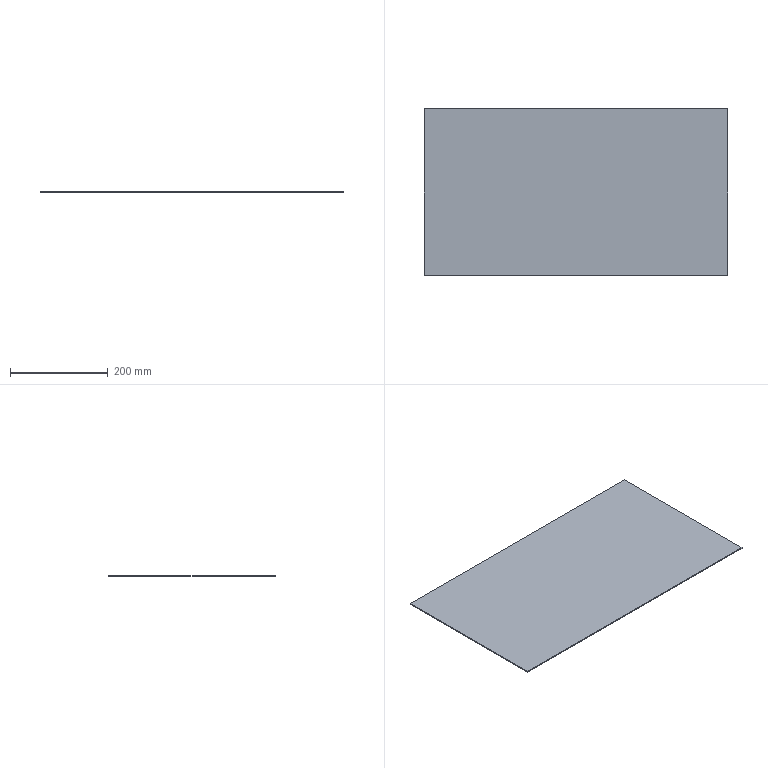Part | SolidWorks | features BaseBody 1 | 1 solid | 6 faces | box 620 x 340 x 2 mm | volume 421600 mm3 | plane 6
STEP:
#1=CARTESIAN_POINT('',(310.,-170.,0.));
#2=VERTEX_POINT('',#1);
#3=CARTESIAN_POINT('',(310.,170.,0.));
#4=VERTEX_POINT('',#3);
#5=CARTESIAN_POINT('',(310.,170.,0.));
#6=DIRECTION('',(0.,1.,0.));
#7=VECTOR('',#6,1000.);
#8=LINE('',#5,#7);
#9=EDGE_CURVE('',#2,#4,#8,.T.);
#10=ORIENTED_EDGE('',*,*,#9,.T.);
#11=CARTESIAN_POINT('',(-310.,170.,0.));
#12=VERTEX_POINT('',#11);
#13=CARTESIAN_POINT('',(-310.,170.,0.));
#14=DIRECTION('',(-1.,0.,0.));
#15=VECTOR('',#14,1000.);
#16=LINE('',#13,#15);
#17=EDGE_CURVE('',#4,#12,#16,.T.);
#18=ORIENTED_EDGE('',*,*,#17,.T.);
#19=CARTESIAN_POINT('',(-310.,-170.,0.));
#20=VERTEX_POINT('',#19);
#21=CARTESIAN_POINT('',(-310.,170.,0.));
#22=DIRECTION('',(0.,-1.,0.));
#23=VECTOR('',#22,1000.);
#24=LINE('',#21,#23);
#25=EDGE_CURVE('',#12,#20,#24,.T.);
#26=ORIENTED_EDGE('',*,*,#25,.T.);
#27=CARTESIAN_POINT('',(-310.,-170.,0.));
#28=DIRECTION('',(1.,0.,0.));
#29=VECTOR('',#28,1000.);
#30=LINE('',#27,#29);
#31=EDGE_CURVE('',#20,#2,#30,.T.);
#32=ORIENTED_EDGE('',*,*,#31,.T.);
#33=EDGE_LOOP('',(#10,#18,#26,#32));
#34=FACE_OUTER_BOUND('',#33,.T.);
#35=CARTESIAN_POINT('',(0.,0.,0.));
#36=DIRECTION('',(0.,0.,1.));
#37=DIRECTION('',(1.,0.,0.));
#38=AXIS2_PLACEMENT_3D('',#35,#36,#37);
#39=PLANE('',#38);
#40=ADVANCED_FACE('',(#34),#39,.T.);
#41=CARTESIAN_POINT('',(310.,-170.,-2.));
#42=VERTEX_POINT('',#41);
#43=CARTESIAN_POINT('',(310.,170.,-2.));
#44=VERTEX_POINT('',#43);
#45=CARTESIAN_POINT('',(310.,170.,-2.));
#46=DIRECTION('',(0.,1.,0.));
#47=VECTOR('',#46,1000.);
#48=LINE('',#45,#47);
#49=EDGE_CURVE('',#42,#44,#48,.T.);
#50=ORIENTED_EDGE('',*,*,#49,.F.);
#51=CARTESIAN_POINT('',(-310.,-170.,-2.));
#52=VERTEX_POINT('',#51);
#53=CARTESIAN_POINT('',(-310.,-170.,-2.));
#54=DIRECTION('',(1.,0.,0.));
#55=VECTOR('',#54,1000.);
#56=LINE('',#53,#55);
#57=EDGE_CURVE('',#52,#42,#56,.T.);
#58=ORIENTED_EDGE('',*,*,#57,.F.);
#59=CARTESIAN_POINT('',(-310.,170.,-2.));
#60=VERTEX_POINT('',#59);
#61=CARTESIAN_POINT('',(-310.,170.,-2.));
#62=DIRECTION('',(0.,-1.,0.));
#63=VECTOR('',#62,1000.);
#64=LINE('',#61,#63);
#65=EDGE_CURVE('',#60,#52,#64,.T.);
#66=ORIENTED_EDGE('',*,*,#65,.F.);
#67=CARTESIAN_POINT('',(-310.,170.,-2.));
#68=DIRECTION('',(-1.,0.,0.));
#69=VECTOR('',#68,1000.);
#70=LINE('',#67,#69);
#71=EDGE_CURVE('',#44,#60,#70,.T.);
#72=ORIENTED_EDGE('',*,*,#71,.F.);
#73=EDGE_LOOP('',(#50,#58,#66,#72));
#74=FACE_OUTER_BOUND('',#73,.T.);
#75=CARTESIAN_POINT('',(0.,0.,-2.));
#76=DIRECTION('',(0.,0.,1.));
#77=DIRECTION('',(1.,0.,0.));
#78=AXIS2_PLACEMENT_3D('',#75,#76,#77);
#79=PLANE('',#78);
#80=ADVANCED_FACE('',(#74),#79,.F.);
#81=ORIENTED_EDGE('',*,*,#17,.F.);
#82=CARTESIAN_POINT('',(310.,170.,-2.));
#83=DIRECTION('',(0.,0.,1.));
#84=VECTOR('',#83,1000.);
#85=LINE('',#82,#84);
#86=EDGE_CURVE('',#44,#4,#85,.T.);
#87=ORIENTED_EDGE('',*,*,#86,.F.);
#88=ORIENTED_EDGE('',*,*,#71,.T.);
#89=CARTESIAN_POINT('',(-310.,170.,-2.));
#90=DIRECTION('',(0.,0.,1.));
#91=VECTOR('',#90,1000.);
#92=LINE('',#89,#91);
#93=EDGE_CURVE('',#60,#12,#92,.T.);
#94=ORIENTED_EDGE('',*,*,#93,.T.);
#95=EDGE_LOOP('',(#81,#87,#88,#94));
#96=FACE_OUTER_BOUND('',#95,.T.);
#97=CARTESIAN_POINT('',(-310.,170.,-2.));
#98=DIRECTION('',(0.,1.,0.));
#99=DIRECTION('',(1.,0.,0.));
#100=AXIS2_PLACEMENT_3D('',#97,#98,#99);
#101=PLANE('',#100);
#102=ADVANCED_FACE('',(#96),#101,.T.);
#103=ORIENTED_EDGE('',*,*,#25,.F.);
#104=ORIENTED_EDGE('',*,*,#93,.F.);
#105=ORIENTED_EDGE('',*,*,#65,.T.);
#106=CARTESIAN_POINT('',(-310.,-170.,-2.));
#107=DIRECTION('',(0.,0.,1.));
#108=VECTOR('',#107,1000.);
#109=LINE('',#106,#108);
#110=EDGE_CURVE('',#52,#20,#109,.T.);
#111=ORIENTED_EDGE('',*,*,#110,.T.);
#112=EDGE_LOOP('',(#103,#104,#105,#111));
#113=FACE_OUTER_BOUND('',#112,.T.);
#114=CARTESIAN_POINT('',(-310.,170.,-2.));
#115=DIRECTION('',(-1.,0.,0.));
#116=DIRECTION('',(0.,1.,0.));
#117=AXIS2_PLACEMENT_3D('',#114,#115,#116);
#118=PLANE('',#117);
#119=ADVANCED_FACE('',(#113),#118,.T.);
#120=ORIENTED_EDGE('',*,*,#31,.F.);
#121=ORIENTED_EDGE('',*,*,#110,.F.);
#122=ORIENTED_EDGE('',*,*,#57,.T.);
#123=CARTESIAN_POINT('',(310.,-170.,-2.));
#124=DIRECTION('',(0.,0.,1.));
#125=VECTOR('',#124,1000.);
#126=LINE('',#123,#125);
#127=EDGE_CURVE('',#42,#2,#126,.T.);
#128=ORIENTED_EDGE('',*,*,#127,.T.);
#129=EDGE_LOOP('',(#120,#121,#122,#128));
#130=FACE_OUTER_BOUND('',#129,.T.);
#131=CARTESIAN_POINT('',(-310.,-170.,-2.));
#132=DIRECTION('',(0.,-1.,0.));
#133=DIRECTION('',(0.,0.,-1.));
#134=AXIS2_PLACEMENT_3D('',#131,#132,#133);
#135=PLANE('',#134);
#136=ADVANCED_FACE('',(#130),#135,.T.);
#137=ORIENTED_EDGE('',*,*,#9,.F.);
#138=ORIENTED_EDGE('',*,*,#127,.F.);
#139=ORIENTED_EDGE('',*,*,#49,.T.);
#140=ORIENTED_EDGE('',*,*,#86,.T.);
#141=EDGE_LOOP('',(#137,#138,#139,#140));
#142=FACE_OUTER_BOUND('',#141,.T.);
#143=CARTESIAN_POINT('',(310.,170.,-2.));
#144=DIRECTION('',(1.,0.,0.));
#145=DIRECTION('',(0.,1.,0.));
#146=AXIS2_PLACEMENT_3D('',#143,#144,#145);
#147=PLANE('',#146);
#148=ADVANCED_FACE('',(#142),#147,.T.);
#149=CLOSED_SHELL('',(#40,#80,#102,#119,#136,#148));
#150=MANIFOLD_SOLID_BREP('',#149);
#151=CARTESIAN_POINT('',(0.,0.,0.));
#152=DIRECTION('',(0.,0.,1.));
#153=DIRECTION('',(1.,0.,0.));
#154=AXIS2_PLACEMENT_3D('',#151,#152,#153);
#155=(LENGTH_UNIT()NAMED_UNIT(*)SI_UNIT(.MILLI.,.METRE.));
#156=UNCERTAINTY_MEASURE_WITH_UNIT(LENGTH_MEASURE(0.00001),#155,'','');
#157=(NAMED_UNIT(*)PLANE_ANGLE_UNIT()SI_UNIT($,.RADIAN.));
#158=(NAMED_UNIT(*)SI_UNIT($,.STERADIAN.)SOLID_ANGLE_UNIT());
#159=(GEOMETRIC_REPRESENTATION_CONTEXT(3)GLOBAL_UNCERTAINTY_ASSIGNED_CONTEXT((#156))GLOBAL_UNIT_ASSIGNED_CONTEXT((#155,#157,#158))REPRESENTATION_CONTEXT('',''));
#160=ADVANCED_BREP_SHAPE_REPRESENTATION('',(#150,#154),#159);